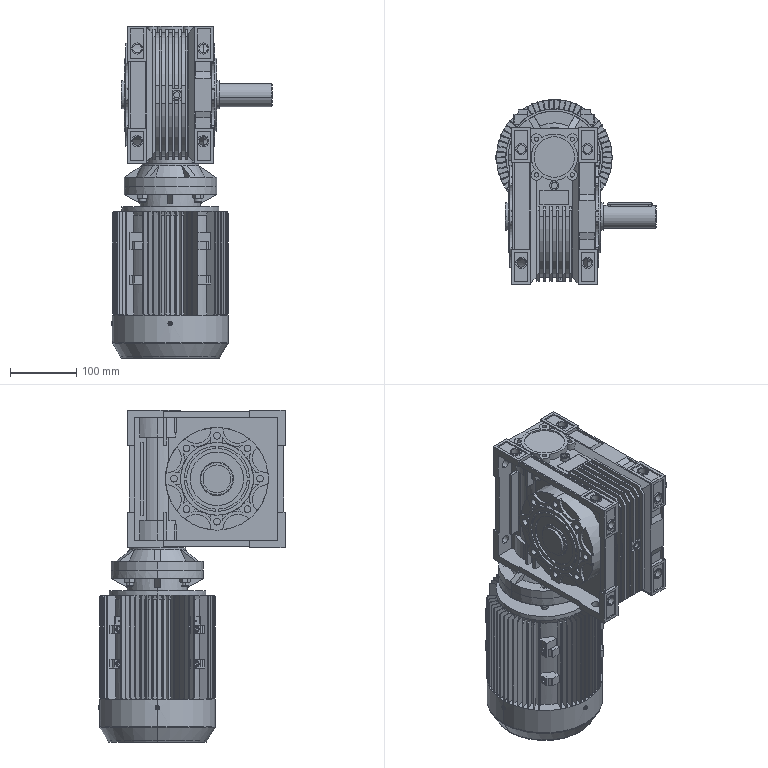Part | SolidWorks | features BaseBody 5 | 5 solids | 2936 faces | box 242.375 x 281.375 x 502 mm | volume 14159606 mm3 | plane 1866 | cylinder 819 | cone 191 | torus 60 | commonest cylinder face diameters 7 x216 143.5 x104 10 x54 45.27 x40 3.6 x36 0.42 x32